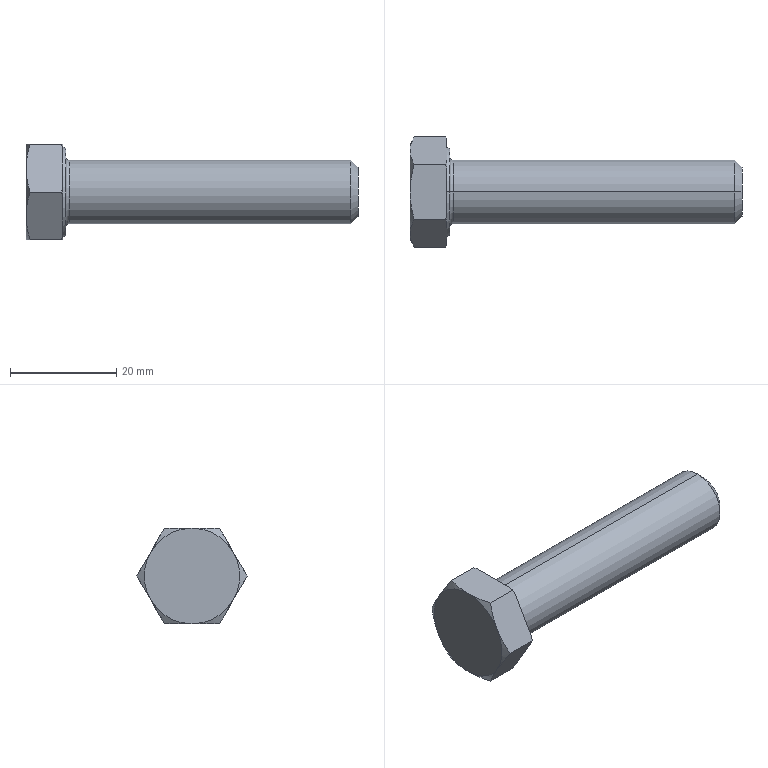Part | SolidWorks | features RevCut 4, Revolution 2, Chamfer 1, Extrusion 1, LPattern 1 | 1 solid | 30 faces | box 62.5 x 20.785 x 18 mm | volume 8250 mm3 | cone 16 | plane 10 | cylinder 2 | torus 2 | commonest cylinder face diameters 12 x2
STEP:
#1=CARTESIAN_POINT('',(8.1,0.,6.));
#2=VERTEX_POINT('',#1);
#3=CARTESIAN_POINT('',(8.1,0.,-6.));
#4=VERTEX_POINT('',#3);
#5=CARTESIAN_POINT('',(8.1,0.,0.));
#6=DIRECTION('',(-1.,0.,0.));
#7=DIRECTION('',(0.,0.,1.));
#8=AXIS2_PLACEMENT_3D('',#5,#6,#7);
#9=CIRCLE('',#8,6.);
#10=EDGE_CURVE('',#2,#4,#9,.T.);
#11=ORIENTED_EDGE('',*,*,#10,.F.);
#12=CARTESIAN_POINT('',(61.1,0.,6.));
#13=VERTEX_POINT('',#12);
#14=CARTESIAN_POINT('',(0.,0.,6.));
#15=DIRECTION('',(1.,0.,0.));
#16=VECTOR('',#15,1000.);
#17=LINE('',#14,#16);
#18=EDGE_CURVE('',#2,#13,#17,.T.);
#19=ORIENTED_EDGE('',*,*,#18,.T.);
#20=CARTESIAN_POINT('',(61.1,0.,-6.));
#21=VERTEX_POINT('',#20);
#22=CARTESIAN_POINT('',(61.1,0.,0.));
#23=DIRECTION('',(-1.,0.,0.));
#24=DIRECTION('',(0.,0.,-1.));
#25=AXIS2_PLACEMENT_3D('',#22,#23,#24);
#26=CIRCLE('',#25,6.);
#27=EDGE_CURVE('',#13,#21,#26,.T.);
#28=ORIENTED_EDGE('',*,*,#27,.T.);
#29=CARTESIAN_POINT('',(0.,0.,-6.));
#30=DIRECTION('',(1.,0.,0.));
#31=VECTOR('',#30,1000.);
#32=LINE('',#29,#31);
#33=EDGE_CURVE('',#4,#21,#32,.T.);
#34=ORIENTED_EDGE('',*,*,#33,.F.);
#35=EDGE_LOOP('',(#11,#19,#28,#34));
#36=FACE_OUTER_BOUND('',#35,.T.);
#37=CARTESIAN_POINT('',(0.,0.,0.));
#38=DIRECTION('',(1.,0.,0.));
#39=DIRECTION('',(0.,0.,-1.));
#40=AXIS2_PLACEMENT_3D('',#37,#38,#39);
#41=CYLINDRICAL_SURFACE('',#40,6.);
#42=ADVANCED_FACE('',(#36),#41,.T.);
#43=CARTESIAN_POINT('',(62.5,0.,-4.6));
#44=VERTEX_POINT('',#43);
#45=CARTESIAN_POINT('',(62.5,0.,4.6));
#46=VERTEX_POINT('',#45);
#47=CARTESIAN_POINT('',(62.5,0.,0.));
#48=DIRECTION('',(1.,0.,0.));
#49=DIRECTION('',(0.,0.,-1.));
#50=AXIS2_PLACEMENT_3D('',#47,#48,#49);
#51=CIRCLE('',#50,4.6);
#52=EDGE_CURVE('',#44,#46,#51,.T.);
#53=ORIENTED_EDGE('',*,*,#52,.F.);
#54=CARTESIAN_POINT('',(62.5,0.,-4.6));
#55=DIRECTION('',(-0.7071,0.,-0.7071));
#56=VECTOR('',#55,1000.);
#57=LINE('',#54,#56);
#58=EDGE_CURVE('',#44,#21,#57,.T.);
#59=ORIENTED_EDGE('',*,*,#58,.T.);
#60=ORIENTED_EDGE('',*,*,#27,.F.);
#61=CARTESIAN_POINT('',(62.5,0.,4.6));
#62=DIRECTION('',(-0.7071,0.,0.7071));
#63=VECTOR('',#62,1000.);
#64=LINE('',#61,#63);
#65=EDGE_CURVE('',#46,#13,#64,.T.);
#66=ORIENTED_EDGE('',*,*,#65,.F.);
#67=EDGE_LOOP('',(#53,#59,#60,#66));
#68=FACE_OUTER_BOUND('',#67,.T.);
#69=CARTESIAN_POINT('',(62.5,0.,0.));
#70=DIRECTION('',(-1.,0.,0.));
#71=DIRECTION('',(0.,0.,1.));
#72=AXIS2_PLACEMENT_3D('',#69,#70,#71);
#73=CONICAL_SURFACE('',#72,4.6,0.7854);
#74=ADVANCED_FACE('',(#68),#73,.T.);
#75=CARTESIAN_POINT('',(7.5,0.,-6.6));
#76=VERTEX_POINT('',#75);
#77=CARTESIAN_POINT('',(7.5,0.,6.6));
#78=VERTEX_POINT('',#77);
#79=CARTESIAN_POINT('',(7.5,0.,0.));
#80=DIRECTION('',(-1.,0.,0.));
#81=DIRECTION('',(0.,0.,1.));
#82=AXIS2_PLACEMENT_3D('',#79,#80,#81);
#83=CIRCLE('',#82,6.6);
#84=EDGE_CURVE('',#76,#78,#83,.T.);
#85=ORIENTED_EDGE('',*,*,#84,.F.);
#86=CARTESIAN_POINT('',(8.1,0.,-6.6));
#87=DIRECTION('',(0.,1.,0.));
#88=DIRECTION('',(-1.,0.,0.));
#89=AXIS2_PLACEMENT_3D('',#86,#87,#88);
#90=CIRCLE('',#89,0.6);
#91=EDGE_CURVE('',#76,#4,#90,.T.);
#92=ORIENTED_EDGE('',*,*,#91,.T.);
#93=CARTESIAN_POINT('',(8.1,0.,0.));
#94=DIRECTION('',(-1.,0.,0.));
#95=DIRECTION('',(0.,0.,1.));
#96=AXIS2_PLACEMENT_3D('',#93,#94,#95);
#97=CIRCLE('',#96,6.);
#98=EDGE_CURVE('',#4,#2,#97,.T.);
#99=ORIENTED_EDGE('',*,*,#98,.T.);
#100=CARTESIAN_POINT('',(8.1,0.,6.6));
#101=DIRECTION('',(0.,-1.,0.));
#102=DIRECTION('',(1.,0.,0.));
#103=AXIS2_PLACEMENT_3D('',#100,#101,#102);
#104=CIRCLE('',#103,0.6);
#105=EDGE_CURVE('',#78,#2,#104,.T.);
#106=ORIENTED_EDGE('',*,*,#105,.F.);
#107=EDGE_LOOP('',(#85,#92,#99,#106));
#108=FACE_OUTER_BOUND('',#107,.T.);
#109=CARTESIAN_POINT('',(8.1,0.,0.));
#110=DIRECTION('',(-1.,0.,0.));
#111=DIRECTION('',(0.,0.,1.));
#112=AXIS2_PLACEMENT_3D('',#109,#110,#111);
#113=TOROIDAL_SURFACE('',#112,6.6,0.6);
#114=ADVANCED_FACE('',(#108),#113,.F.);
#115=CARTESIAN_POINT('',(7.5,0.,8.177));
#116=VERTEX_POINT('',#115);
#117=CARTESIAN_POINT('',(7.5,0.,-8.177));
#118=VERTEX_POINT('',#117);
#119=CARTESIAN_POINT('',(7.5,0.,0.));
#120=DIRECTION('',(-1.,0.,0.));
#121=DIRECTION('',(0.,0.,1.));
#122=AXIS2_PLACEMENT_3D('',#119,#120,#121);
#123=CIRCLE('',#122,8.177);
#124=EDGE_CURVE('',#116,#118,#123,.T.);
#125=ORIENTED_EDGE('',*,*,#124,.T.);
#126=CARTESIAN_POINT('',(6.9,0.,-8.524));
#127=VERTEX_POINT('',#126);
#128=CARTESIAN_POINT('',(6.9,0.,-8.524));
#129=DIRECTION('',(-0.866,0.,-0.5));
#130=VECTOR('',#129,1000.);
#131=LINE('',#128,#130);
#132=EDGE_CURVE('',#118,#127,#131,.T.);
#133=ORIENTED_EDGE('',*,*,#132,.T.);
#134=CARTESIAN_POINT('',(6.9,0.,8.524));
#135=VERTEX_POINT('',#134);
#136=CARTESIAN_POINT('',(6.9,0.,0.));
#137=DIRECTION('',(-1.,0.,0.));
#138=DIRECTION('',(0.,0.,1.));
#139=AXIS2_PLACEMENT_3D('',#136,#137,#138);
#140=CIRCLE('',#139,8.524);
#141=EDGE_CURVE('',#135,#127,#140,.T.);
#142=ORIENTED_EDGE('',*,*,#141,.F.);
#143=CARTESIAN_POINT('',(6.9,0.,8.524));
#144=DIRECTION('',(-0.866,0.,0.5));
#145=VECTOR('',#144,1000.);
#146=LINE('',#143,#145);
#147=EDGE_CURVE('',#116,#135,#146,.T.);
#148=ORIENTED_EDGE('',*,*,#147,.F.);
#149=EDGE_LOOP('',(#125,#133,#142,#148));
#150=FACE_OUTER_BOUND('',#149,.T.);
#151=CARTESIAN_POINT('',(6.9,0.,0.));
#152=DIRECTION('',(-1.,0.,0.));
#153=DIRECTION('',(0.,0.,1.));
#154=AXIS2_PLACEMENT_3D('',#151,#152,#153);
#155=CONICAL_SURFACE('',#154,8.524,0.5236);
#156=ADVANCED_FACE('',(#150),#155,.T.);
#157=ORIENTED_EDGE('',*,*,#124,.F.);
#158=CARTESIAN_POINT('',(7.5,0.,0.));
#159=DIRECTION('',(-1.,0.,0.));
#160=DIRECTION('',(0.,0.,1.));
#161=AXIS2_PLACEMENT_3D('',#158,#159,#160);
#162=CIRCLE('',#161,8.177);
#163=EDGE_CURVE('',#118,#116,#162,.T.);
#164=ORIENTED_EDGE('',*,*,#163,.F.);
#165=EDGE_LOOP('',(#157,#164));
#166=FACE_OUTER_BOUND('',#165,.T.);
#167=CARTESIAN_POINT('',(7.5,0.,0.));
#168=DIRECTION('',(-1.,0.,0.));
#169=DIRECTION('',(0.,0.,1.));
#170=AXIS2_PLACEMENT_3D('',#167,#168,#169);
#171=CIRCLE('',#170,6.6);
#172=EDGE_CURVE('',#78,#76,#171,.T.);
#173=ORIENTED_EDGE('',*,*,#172,.T.);
#174=ORIENTED_EDGE('',*,*,#84,.T.);
#175=EDGE_LOOP('',(#173,#174));
#176=FACE_BOUND('',#175,.T.);
#177=CARTESIAN_POINT('',(7.5,0.,-18.));
#178=DIRECTION('',(1.,0.,0.));
#179=DIRECTION('',(0.,0.,-1.));
#180=AXIS2_PLACEMENT_3D('',#177,#178,#179);
#181=PLANE('',#180);
#182=ADVANCED_FACE('',(#166,#176),#181,.T.);
#183=CARTESIAN_POINT('',(6.9,5.57,-8.352));
#184=VERTEX_POINT('',#183);
#185=CARTESIAN_POINT('',(6.9,10.018,-0.6478));
#186=VERTEX_POINT('',#185);
#187=CARTESIAN_POINT('',(6.9,5.196,-9.));
#188=DIRECTION('',(0.,0.5,0.866));
#189=VECTOR('',#188,1000.);
#190=LINE('',#187,#189);
#191=EDGE_CURVE('',#184,#186,#190,.T.);
#192=ORIENTED_EDGE('',*,*,#191,.F.);
#193=CARTESIAN_POINT('',(6.696,5.196,-9.));
#194=VERTEX_POINT('',#193);
#195=CARTESIAN_POINT('',(6.696,5.196,-9.));
#196=CARTESIAN_POINT('',(6.768,5.321,-8.785));
#197=CARTESIAN_POINT('',(6.836,5.445,-8.569));
#198=CARTESIAN_POINT('',(6.9,5.57,-8.352));
#199=B_SPLINE_CURVE_WITH_KNOTS('',3,(#195,#196,#197,#198),.UNSPECIFIED.,.F.,.F.,(4,4),(0.000000238,0.0007696),.UNSPECIFIED.);
#200=EDGE_CURVE('',#194,#184,#199,.T.);
#201=ORIENTED_EDGE('',*,*,#200,.F.);
#202=CARTESIAN_POINT('',(0.8038,5.196,-9.));
#203=VERTEX_POINT('',#202);
#204=CARTESIAN_POINT('',(7.5,5.196,-9.));
#205=DIRECTION('',(-1.,0.,0.));
#206=VECTOR('',#205,1000.);
#207=LINE('',#204,#206);
#208=EDGE_CURVE('',#194,#203,#207,.T.);
#209=ORIENTED_EDGE('',*,*,#208,.T.);
#210=CARTESIAN_POINT('',(0.,7.794,-4.5));
#211=VERTEX_POINT('',#210);
#212=CARTESIAN_POINT('',(0.,7.794,-4.5));
#213=CARTESIAN_POINT('',(0.,7.574,-4.882));
#214=CARTESIAN_POINT('',(0.019,7.352,-5.266));
#215=CARTESIAN_POINT('',(0.09253,6.914,-6.024));
#216=CARTESIAN_POINT('',(0.147,6.697,-6.401));
#217=CARTESIAN_POINT('',(0.357,6.048,-7.525));
#218=CARTESIAN_POINT('',(0.5591,5.62,-8.266));
#219=CARTESIAN_POINT('',(0.8038,5.196,-9.));
#220=B_SPLINE_CURVE_WITH_KNOTS('',3,(#212,#213,#214,#215,#216,#217,#218,#219),.UNSPECIFIED.,.F.,.F.,(4,2,2,4),(0.005258,0.006567,0.007877,0.0105),.UNSPECIFIED.);
#221=EDGE_CURVE('',#211,#203,#220,.T.);
#222=ORIENTED_EDGE('',*,*,#221,.F.);
#223=CARTESIAN_POINT('',(0.8038,10.392,0.));
#224=VERTEX_POINT('',#223);
#225=CARTESIAN_POINT('',(0.8038,10.392,0.));
#226=CARTESIAN_POINT('',(0.5585,9.967,-0.7361));
#227=CARTESIAN_POINT('',(0.3563,9.539,-1.478));
#228=CARTESIAN_POINT('',(0.07661,8.674,-2.976));
#229=CARTESIAN_POINT('',(0.,8.237,-3.733));
#230=CARTESIAN_POINT('',(0.,7.794,-4.5));
#231=B_SPLINE_CURVE_WITH_KNOTS('',3,(#225,#226,#227,#228,#229,#230),.UNSPECIFIED.,.F.,.F.,(4,2,4),(0.000000238,0.002629,0.005258),.UNSPECIFIED.);
#232=EDGE_CURVE('',#224,#211,#231,.T.);
#233=ORIENTED_EDGE('',*,*,#232,.F.);
#234=CARTESIAN_POINT('',(6.696,10.392,0.));
#235=VERTEX_POINT('',#234);
#236=CARTESIAN_POINT('',(7.5,10.392,0.));
#237=DIRECTION('',(-1.,0.,0.));
#238=VECTOR('',#237,1000.);
#239=LINE('',#236,#238);
#240=EDGE_CURVE('',#235,#224,#239,.T.);
#241=ORIENTED_EDGE('',*,*,#240,.F.);
#242=CARTESIAN_POINT('',(6.9,10.018,-0.6478));
#243=CARTESIAN_POINT('',(6.836,10.143,-0.4313));
#244=CARTESIAN_POINT('',(6.768,10.268,-0.2154));
#245=CARTESIAN_POINT('',(6.696,10.392,0.));
#246=B_SPLINE_CURVE_WITH_KNOTS('',3,(#242,#243,#244,#245),.UNSPECIFIED.,.F.,.F.,(4,4),(0.009728,0.0105),.UNSPECIFIED.);
#247=EDGE_CURVE('',#186,#235,#246,.T.);
#248=ORIENTED_EDGE('',*,*,#247,.F.);
#249=EDGE_LOOP('',(#192,#201,#209,#222,#233,#241,#248));
#250=FACE_OUTER_BOUND('',#249,.T.);
#251=CARTESIAN_POINT('',(7.5,5.196,-9.));
#252=DIRECTION('',(0.,-0.866,0.5));
#253=DIRECTION('',(0.,-0.5,-0.866));
#254=AXIS2_PLACEMENT_3D('',#251,#252,#253);
#255=PLANE('',#254);
#256=ADVANCED_FACE('',(#250),#255,.F.);
#257=CARTESIAN_POINT('',(6.9,10.018,0.6478));
#258=VERTEX_POINT('',#257);
#259=CARTESIAN_POINT('',(6.9,5.57,8.352));
#260=VERTEX_POINT('',#259);
#261=CARTESIAN_POINT('',(6.9,10.392,0.));
#262=DIRECTION('',(0.,-0.5,0.866));
#263=VECTOR('',#262,1000.);
#264=LINE('',#261,#263);
#265=EDGE_CURVE('',#258,#260,#264,.T.);
#266=ORIENTED_EDGE('',*,*,#265,.F.);
#267=CARTESIAN_POINT('',(6.696,10.392,0.));
#268=CARTESIAN_POINT('',(6.768,10.268,0.2154));
#269=CARTESIAN_POINT('',(6.836,10.143,0.4314));
#270=CARTESIAN_POINT('',(6.9,10.018,0.6478));
#271=B_SPLINE_CURVE_WITH_KNOTS('',3,(#267,#268,#269,#270),.UNSPECIFIED.,.F.,.F.,(4,4),(0.000000238,0.0007696),.UNSPECIFIED.);
#272=EDGE_CURVE('',#235,#258,#271,.T.);
#273=ORIENTED_EDGE('',*,*,#272,.F.);
#274=ORIENTED_EDGE('',*,*,#240,.T.);
#275=CARTESIAN_POINT('',(0.,7.794,4.5));
#276=VERTEX_POINT('',#275);
#277=CARTESIAN_POINT('',(0.,7.794,4.5));
#278=CARTESIAN_POINT('',(0.,8.015,4.118));
#279=CARTESIAN_POINT('',(0.019,8.236,3.734));
#280=CARTESIAN_POINT('',(0.09253,8.674,2.976));
#281=CARTESIAN_POINT('',(0.147,8.892,2.599));
#282=CARTESIAN_POINT('',(0.357,9.541,1.475));
#283=CARTESIAN_POINT('',(0.5591,9.968,0.7343));
#284=CARTESIAN_POINT('',(0.8038,10.392,0.));
#285=B_SPLINE_CURVE_WITH_KNOTS('',3,(#277,#278,#279,#280,#281,#282,#283,#284),.UNSPECIFIED.,.F.,.F.,(4,2,2,4),(0.005258,0.006567,0.007877,0.0105),.UNSPECIFIED.);
#286=EDGE_CURVE('',#276,#224,#285,.T.);
#287=ORIENTED_EDGE('',*,*,#286,.F.);
#288=CARTESIAN_POINT('',(0.8038,5.196,9.));
#289=VERTEX_POINT('',#288);
#290=CARTESIAN_POINT('',(0.8038,5.196,9.));
#291=CARTESIAN_POINT('',(0.5585,5.621,8.264));
#292=CARTESIAN_POINT('',(0.3563,6.049,7.522));
#293=CARTESIAN_POINT('',(0.07661,6.914,6.024));
#294=CARTESIAN_POINT('',(0.,7.352,5.267));
#295=CARTESIAN_POINT('',(0.,7.794,4.5));
#296=B_SPLINE_CURVE_WITH_KNOTS('',3,(#290,#291,#292,#293,#294,#295),.UNSPECIFIED.,.F.,.F.,(4,2,4),(0.000000238,0.002629,0.005258),.UNSPECIFIED.);
#297=EDGE_CURVE('',#289,#276,#296,.T.);
#298=ORIENTED_EDGE('',*,*,#297,.F.);
#299=CARTESIAN_POINT('',(6.696,5.196,9.));
#300=VERTEX_POINT('',#299);
#301=CARTESIAN_POINT('',(7.5,5.196,9.));
#302=DIRECTION('',(-1.,0.,0.));
#303=VECTOR('',#302,1000.);
#304=LINE('',#301,#303);
#305=EDGE_CURVE('',#300,#289,#304,.T.);
#306=ORIENTED_EDGE('',*,*,#305,.F.);
#307=CARTESIAN_POINT('',(6.9,5.57,8.352));
#308=CARTESIAN_POINT('',(6.836,5.445,8.569));
#309=CARTESIAN_POINT('',(6.768,5.32,8.785));
#310=CARTESIAN_POINT('',(6.696,5.196,9.));
#311=B_SPLINE_CURVE_WITH_KNOTS('',3,(#307,#308,#309,#310),.UNSPECIFIED.,.F.,.F.,(4,4),(0.009728,0.0105),.UNSPECIFIED.);
#312=EDGE_CURVE('',#260,#300,#311,.T.);
#313=ORIENTED_EDGE('',*,*,#312,.F.);
#314=EDGE_LOOP('',(#266,#273,#274,#287,#298,#306,#313));
#315=FACE_OUTER_BOUND('',#314,.T.);
#316=CARTESIAN_POINT('',(7.5,10.392,0.));
#317=DIRECTION('',(0.,-0.866,-0.5));
#318=DIRECTION('',(0.,0.5,-0.866));
#319=AXIS2_PLACEMENT_3D('',#316,#317,#318);
#320=PLANE('',#319);
#321=ADVANCED_FACE('',(#315),#320,.F.);
#322=CARTESIAN_POINT('',(6.9,4.448,9.));
#323=VERTEX_POINT('',#322);
#324=CARTESIAN_POINT('',(6.9,-4.448,9.));
#325=VERTEX_POINT('',#324);
#326=CARTESIAN_POINT('',(6.9,5.196,9.));
#327=DIRECTION('',(0.,-1.,0.));
#328=VECTOR('',#327,1000.);
#329=LINE('',#326,#328);
#330=EDGE_CURVE('',#323,#325,#329,.T.);
#331=ORIENTED_EDGE('',*,*,#330,.F.);
#332=CARTESIAN_POINT('',(6.696,5.196,9.));
#333=CARTESIAN_POINT('',(6.768,4.948,9.));
#334=CARTESIAN_POINT('',(6.836,4.698,9.));
#335=CARTESIAN_POINT('',(6.9,4.448,9.));
#336=B_SPLINE_CURVE_WITH_KNOTS('',3,(#332,#333,#334,#335),.UNSPECIFIED.,.F.,.F.,(4,4),(0.02519,0.02597),.UNSPECIFIED.);
#337=EDGE_CURVE('',#300,#323,#336,.T.);
#338=ORIENTED_EDGE('',*,*,#337,.F.);
#339=ORIENTED_EDGE('',*,*,#305,.T.);
#340=CARTESIAN_POINT('',(0.,0.,9.));
#341=VERTEX_POINT('',#340);
#342=CARTESIAN_POINT('',(0.,0.,9.));
#343=CARTESIAN_POINT('',(0.,0.4401,9.));
#344=CARTESIAN_POINT('',(0.01885,0.8832,9.));
#345=CARTESIAN_POINT('',(0.09319,1.767,9.));
#346=CARTESIAN_POINT('',(0.1482,2.204,9.));
#347=CARTESIAN_POINT('',(0.3593,3.505,9.));
#348=CARTESIAN_POINT('',(0.5612,4.356,9.));
#349=CARTESIAN_POINT('',(0.8038,5.196,9.));
#350=B_SPLINE_CURVE_WITH_KNOTS('',3,(#342,#343,#344,#345,#346,#347,#348,#349),.UNSPECIFIED.,.F.,.F.,(4,2,2,4),(0.01498,0.0163,0.01761,0.02025),.UNSPECIFIED.);
#351=EDGE_CURVE('',#341,#289,#350,.T.);
#352=ORIENTED_EDGE('',*,*,#351,.F.);
#353=CARTESIAN_POINT('',(0.8038,-5.196,9.));
#354=VERTEX_POINT('',#353);
#355=CARTESIAN_POINT('',(0.8038,-5.196,9.));
#356=CARTESIAN_POINT('',(0.5595,-4.35,9.));
#357=CARTESIAN_POINT('',(0.3552,-3.485,9.));
#358=CARTESIAN_POINT('',(0.07569,-1.752,9.));
#359=CARTESIAN_POINT('',(0.,-0.8794,9.));
#360=CARTESIAN_POINT('',(0.,0.,9.));
#361=B_SPLINE_CURVE_WITH_KNOTS('',3,(#355,#356,#357,#358,#359,#360),.UNSPECIFIED.,.F.,.F.,(4,2,4),(0.00972,0.01235,0.01498),.UNSPECIFIED.);
#362=EDGE_CURVE('',#354,#341,#361,.T.);
#363=ORIENTED_EDGE('',*,*,#362,.F.);
#364=CARTESIAN_POINT('',(6.696,-5.196,9.));
#365=VERTEX_POINT('',#364);
#366=CARTESIAN_POINT('',(7.5,-5.196,9.));
#367=DIRECTION('',(-1.,0.,0.));
#368=VECTOR('',#367,1000.);
#369=LINE('',#366,#368);
#370=EDGE_CURVE('',#365,#354,#369,.T.);
#371=ORIENTED_EDGE('',*,*,#370,.F.);
#372=CARTESIAN_POINT('',(6.9,-4.448,9.));
#373=CARTESIAN_POINT('',(6.836,-4.699,9.));
#374=CARTESIAN_POINT('',(6.768,-4.948,9.));
#375=CARTESIAN_POINT('',(6.696,-5.196,9.));
#376=B_SPLINE_CURVE_WITH_KNOTS('',3,(#372,#373,#374,#375),.UNSPECIFIED.,.F.,.F.,(4,4),(0.03494,0.03571),.UNSPECIFIED.);
#377=EDGE_CURVE('',#325,#365,#376,.T.);
#378=ORIENTED_EDGE('',*,*,#377,.F.);
#379=EDGE_LOOP('',(#331,#338,#339,#352,#363,#371,#378));
#380=FACE_OUTER_BOUND('',#379,.T.);
#381=CARTESIAN_POINT('',(7.5,5.196,9.));
#382=DIRECTION('',(0.,0.,-1.));
#383=DIRECTION('',(0.,1.,0.));
#384=AXIS2_PLACEMENT_3D('',#381,#382,#383);
#385=PLANE('',#384);
#386=ADVANCED_FACE('',(#380),#385,.F.);
#387=CARTESIAN_POINT('',(6.9,-5.57,8.352));
#388=VERTEX_POINT('',#387);
#389=CARTESIAN_POINT('',(6.9,-10.018,0.6478));
#390=VERTEX_POINT('',#389);
#391=CARTESIAN_POINT('',(6.9,-10.392,0.));
#392=DIRECTION('',(0.,-0.5,-0.866));
#393=VECTOR('',#392,1000.);
#394=LINE('',#391,#393);
#395=EDGE_CURVE('',#388,#390,#394,.T.);
#396=ORIENTED_EDGE('',*,*,#395,.F.);
#397=CARTESIAN_POINT('',(6.696,-5.196,9.));
#398=CARTESIAN_POINT('',(6.768,-5.321,8.785));
#399=CARTESIAN_POINT('',(6.836,-5.445,8.569));
#400=CARTESIAN_POINT('',(6.9,-5.57,8.352));
#401=B_SPLINE_CURVE_WITH_KNOTS('',3,(#397,#398,#399,#400),.UNSPECIFIED.,.F.,.F.,(4,4),(0.000000238,0.0007696),.UNSPECIFIED.);
#402=EDGE_CURVE('',#365,#388,#401,.T.);
#403=ORIENTED_EDGE('',*,*,#402,.F.);
#404=ORIENTED_EDGE('',*,*,#370,.T.);
#405=CARTESIAN_POINT('',(0.,-7.794,4.5));
#406=VERTEX_POINT('',#405);
#407=CARTESIAN_POINT('',(0.,-7.794,4.5));
#408=CARTESIAN_POINT('',(0.,-7.574,4.882));
#409=CARTESIAN_POINT('',(0.019,-7.352,5.266));
#410=CARTESIAN_POINT('',(0.09253,-6.914,6.024));
#411=CARTESIAN_POINT('',(0.147,-6.697,6.401));
#412=CARTESIAN_POINT('',(0.357,-6.048,7.525));
#413=CARTESIAN_POINT('',(0.5591,-5.62,8.266));
#414=CARTESIAN_POINT('',(0.8038,-5.196,9.));
#415=B_SPLINE_CURVE_WITH_KNOTS('',3,(#407,#408,#409,#410,#411,#412,#413,#414),.UNSPECIFIED.,.F.,.F.,(4,2,2,4),(0.005258,0.006567,0.007877,0.0105),.UNSPECIFIED.);
#416=EDGE_CURVE('',#406,#354,#415,.T.);
#417=ORIENTED_EDGE('',*,*,#416,.F.);
#418=CARTESIAN_POINT('',(0.8038,-10.392,0.));
#419=VERTEX_POINT('',#418);
#420=CARTESIAN_POINT('',(0.8038,-10.392,0.));
#421=CARTESIAN_POINT('',(0.5585,-9.967,0.7361));
#422=CARTESIAN_POINT('',(0.3563,-9.539,1.478));
#423=CARTESIAN_POINT('',(0.07661,-8.674,2.976));
#424=CARTESIAN_POINT('',(0.,-8.237,3.733));
#425=CARTESIAN_POINT('',(0.,-7.794,4.5));
#426=B_SPLINE_CURVE_WITH_KNOTS('',3,(#420,#421,#422,#423,#424,#425),.UNSPECIFIED.,.F.,.F.,(4,2,4),(0.000000238,0.002629,0.005258),.UNSPECIFIED.);
#427=EDGE_CURVE('',#419,#406,#426,.T.);
#428=ORIENTED_EDGE('',*,*,#427,.F.);
#429=CARTESIAN_POINT('',(6.696,-10.392,0.));
#430=VERTEX_POINT('',#429);
#431=CARTESIAN_POINT('',(7.5,-10.392,0.));
#432=DIRECTION('',(-1.,0.,0.));
#433=VECTOR('',#432,1000.);
#434=LINE('',#431,#433);
#435=EDGE_CURVE('',#430,#419,#434,.T.);
#436=ORIENTED_EDGE('',*,*,#435,.F.);
#437=CARTESIAN_POINT('',(6.9,-10.018,0.6478));
#438=CARTESIAN_POINT('',(6.836,-10.143,0.4313));
#439=CARTESIAN_POINT('',(6.768,-10.268,0.2154));
#440=CARTESIAN_POINT('',(6.696,-10.392,0.));
#441=B_SPLINE_CURVE_WITH_KNOTS('',3,(#437,#438,#439,#440),.UNSPECIFIED.,.F.,.F.,(4,4),(0.009728,0.0105),.UNSPECIFIED.);
#442=EDGE_CURVE('',#390,#430,#441,.T.);
#443=ORIENTED_EDGE('',*,*,#442,.F.);
#444=EDGE_LOOP('',(#396,#403,#404,#417,#428,#436,#443));
#445=FACE_OUTER_BOUND('',#444,.T.);
#446=CARTESIAN_POINT('',(7.5,-10.392,0.));
#447=DIRECTION('',(0.,0.866,-0.5));
#448=DIRECTION('',(0.,0.5,0.866));
#449=AXIS2_PLACEMENT_3D('',#446,#447,#448);
#450=PLANE('',#449);
#451=ADVANCED_FACE('',(#445),#450,.F.);
#452=CARTESIAN_POINT('',(6.9,-10.018,-0.6478));
#453=VERTEX_POINT('',#452);
#454=CARTESIAN_POINT('',(6.9,-5.57,-8.352));
#455=VERTEX_POINT('',#454);
#456=CARTESIAN_POINT('',(6.9,-5.196,-9.));
#457=DIRECTION('',(0.,0.5,-0.866));
#458=VECTOR('',#457,1000.);
#459=LINE('',#456,#458);
#460=EDGE_CURVE('',#453,#455,#459,.T.);
#461=ORIENTED_EDGE('',*,*,#460,.F.);
#462=CARTESIAN_POINT('',(6.696,-10.392,0.));
#463=CARTESIAN_POINT('',(6.768,-10.268,-0.2154));
#464=CARTESIAN_POINT('',(6.836,-10.143,-0.4314));
#465=CARTESIAN_POINT('',(6.9,-10.018,-0.6478));
#466=B_SPLINE_CURVE_WITH_KNOTS('',3,(#462,#463,#464,#465),.UNSPECIFIED.,.F.,.F.,(4,4),(0.000000238,0.0007696),.UNSPECIFIED.);
#467=EDGE_CURVE('',#430,#453,#466,.T.);
#468=ORIENTED_EDGE('',*,*,#467,.F.);
#469=ORIENTED_EDGE('',*,*,#435,.T.);
#470=CARTESIAN_POINT('',(0.,-7.794,-4.5));
#471=VERTEX_POINT('',#470);
#472=CARTESIAN_POINT('',(0.,-7.794,-4.5));
#473=CARTESIAN_POINT('',(0.,-8.015,-4.118));
#474=CARTESIAN_POINT('',(0.019,-8.236,-3.734));
#475=CARTESIAN_POINT('',(0.09253,-8.674,-2.976));
#476=CARTESIAN_POINT('',(0.147,-8.892,-2.599));
#477=CARTESIAN_POINT('',(0.357,-9.541,-1.475));
#478=CARTESIAN_POINT('',(0.5591,-9.968,-0.7343));
#479=CARTESIAN_POINT('',(0.8038,-10.392,0.));
#480=B_SPLINE_CURVE_WITH_KNOTS('',3,(#472,#473,#474,#475,#476,#477,#478,#479),.UNSPECIFIED.,.F.,.F.,(4,2,2,4),(0.005258,0.006567,0.007877,0.0105),.UNSPECIFIED.);
#481=EDGE_CURVE('',#471,#419,#480,.T.);
#482=ORIENTED_EDGE('',*,*,#481,.F.);
#483=CARTESIAN_POINT('',(0.8038,-5.196,-9.));
#484=VERTEX_POINT('',#483);
#485=CARTESIAN_POINT('',(0.8038,-5.196,-9.));
#486=CARTESIAN_POINT('',(0.5585,-5.621,-8.264));
#487=CARTESIAN_POINT('',(0.3563,-6.049,-7.522));
#488=CARTESIAN_POINT('',(0.07661,-6.914,-6.024));
#489=CARTESIAN_POINT('',(0.,-7.352,-5.267));
#490=CARTESIAN_POINT('',(0.,-7.794,-4.5));
#491=B_SPLINE_CURVE_WITH_KNOTS('',3,(#485,#486,#487,#488,#489,#490),.UNSPECIFIED.,.F.,.F.,(4,2,4),(0.000000238,0.002629,0.005258),.UNSPECIFIED.);
#492=EDGE_CURVE('',#484,#471,#491,.T.);
#493=ORIENTED_EDGE('',*,*,#492,.F.);
#494=CARTESIAN_POINT('',(6.696,-5.196,-9.));
#495=VERTEX_POINT('',#494);
#496=CARTESIAN_POINT('',(7.5,-5.196,-9.));
#497=DIRECTION('',(-1.,0.,0.));
#498=VECTOR('',#497,1000.);
#499=LINE('',#496,#498);
#500=EDGE_CURVE('',#495,#484,#499,.T.);
#501=ORIENTED_EDGE('',*,*,#500,.F.);
#502=CARTESIAN_POINT('',(6.9,-5.57,-8.352));
#503=CARTESIAN_POINT('',(6.836,-5.445,-8.569));
#504=CARTESIAN_POINT('',(6.768,-5.32,-8.785));
#505=CARTESIAN_POINT('',(6.696,-5.196,-9.));
#506=B_SPLINE_CURVE_WITH_KNOTS('',3,(#502,#503,#504,#505),.UNSPECIFIED.,.F.,.F.,(4,4),(0.009728,0.0105),.UNSPECIFIED.);
#507=EDGE_CURVE('',#455,#495,#506,.T.);
#508=ORIENTED_EDGE('',*,*,#507,.F.);
#509=EDGE_LOOP('',(#461,#468,#469,#482,#493,#501,#508));
#510=FACE_OUTER_BOUND('',#509,.T.);
#511=CARTESIAN_POINT('',(7.5,-5.196,-9.));
#512=DIRECTION('',(0.,0.866,0.5));
#513=DIRECTION('',(0.,-0.5,0.866));
#514=AXIS2_PLACEMENT_3D('',#511,#512,#513);
#515=PLANE('',#514);
#516=ADVANCED_FACE('',(#510),#515,.F.);
#517=CARTESIAN_POINT('',(6.9,-4.448,-9.));
#518=VERTEX_POINT('',#517);
#519=CARTESIAN_POINT('',(6.9,4.448,-9.));
#520=VERTEX_POINT('',#519);
#521=CARTESIAN_POINT('',(6.9,5.196,-9.));
#522=DIRECTION('',(0.,1.,0.));
#523=VECTOR('',#522,1000.);
#524=LINE('',#521,#523);
#525=EDGE_CURVE('',#518,#520,#524,.T.);
#526=ORIENTED_EDGE('',*,*,#525,.F.);
#527=CARTESIAN_POINT('',(6.696,-5.196,-9.));
#528=CARTESIAN_POINT('',(6.768,-4.948,-9.));
#529=CARTESIAN_POINT('',(6.836,-4.699,-9.));
#530=CARTESIAN_POINT('',(6.9,-4.448,-9.));
#531=B_SPLINE_CURVE_WITH_KNOTS('',3,(#527,#528,#529,#530),.UNSPECIFIED.,.F.,.F.,(4,4),(0.00972,0.01049),.UNSPECIFIED.);
#532=EDGE_CURVE('',#495,#518,#531,.T.);
#533=ORIENTED_EDGE('',*,*,#532,.F.);
#534=ORIENTED_EDGE('',*,*,#500,.T.);
#535=CARTESIAN_POINT('',(0.,0.,-9.));
#536=VERTEX_POINT('',#535);
#537=CARTESIAN_POINT('',(0.,0.,-9.));
#538=CARTESIAN_POINT('',(0.,-0.8794,-9.));
#539=CARTESIAN_POINT('',(0.07569,-1.752,-9.));
#540=CARTESIAN_POINT('',(0.3552,-3.485,-9.));
#541=CARTESIAN_POINT('',(0.5595,-4.35,-9.));
#542=CARTESIAN_POINT('',(0.8038,-5.196,-9.));
#543=B_SPLINE_CURVE_WITH_KNOTS('',3,(#537,#538,#539,#540,#541,#542),.UNSPECIFIED.,.F.,.F.,(4,2,4),(0.03045,0.03308,0.03571),.UNSPECIFIED.);
#544=EDGE_CURVE('',#536,#484,#543,.T.);
#545=ORIENTED_EDGE('',*,*,#544,.F.);
#546=CARTESIAN_POINT('',(0.8038,5.196,-9.));
#547=CARTESIAN_POINT('',(0.5612,4.356,-9.));
#548=CARTESIAN_POINT('',(0.3593,3.505,-9.));
#549=CARTESIAN_POINT('',(0.1482,2.204,-9.));
#550=CARTESIAN_POINT('',(0.09319,1.767,-9.));
#551=CARTESIAN_POINT('',(0.01885,0.8832,-9.));
#552=CARTESIAN_POINT('',(0.,0.4401,-9.));
#553=CARTESIAN_POINT('',(0.,0.,-9.));
#554=B_SPLINE_CURVE_WITH_KNOTS('',3,(#546,#547,#548,#549,#550,#551,#552,#553),.UNSPECIFIED.,.F.,.F.,(4,2,2,4),(0.02519,0.02782,0.02914,0.03045),.UNSPECIFIED.);
#555=EDGE_CURVE('',#203,#536,#554,.T.);
#556=ORIENTED_EDGE('',*,*,#555,.F.);
#557=ORIENTED_EDGE('',*,*,#208,.F.);
#558=CARTESIAN_POINT('',(6.9,4.448,-9.));
#559=CARTESIAN_POINT('',(6.836,4.698,-9.));
#560=CARTESIAN_POINT('',(6.768,4.948,-9.));
#561=CARTESIAN_POINT('',(6.696,5.196,-9.));
#562=B_SPLINE_CURVE_WITH_KNOTS('',3,(#558,#559,#560,#561),.UNSPECIFIED.,.F.,.F.,(4,4),(0.01947,0.02025),.UNSPECIFIED.);
#563=EDGE_CURVE('',#520,#194,#562,.T.);
#564=ORIENTED_EDGE('',*,*,#563,.F.);
#565=EDGE_LOOP('',(#526,#533,#534,#545,#556,#557,#564));
#566=FACE_OUTER_BOUND('',#565,.T.);
#567=CARTESIAN_POINT('',(7.5,5.196,-9.));
#568=DIRECTION('',(0.,0.,1.));
#569=DIRECTION('',(0.,-1.,0.));
#570=AXIS2_PLACEMENT_3D('',#567,#568,#569);
#571=PLANE('',#570);
#572=ADVANCED_FACE('',(#566),#571,.F.);
#573=ORIENTED_EDGE('',*,*,#532,.T.);
#574=CARTESIAN_POINT('',(6.9,0.,0.));
#575=DIRECTION('',(-1.,0.,0.));
#576=DIRECTION('',(0.,0.,-1.));
#577=AXIS2_PLACEMENT_3D('',#574,#575,#576);
#578=CIRCLE('',#577,10.039);
#579=EDGE_CURVE('',#518,#455,#578,.T.);
#580=ORIENTED_EDGE('',*,*,#579,.T.);
#581=ORIENTED_EDGE('',*,*,#507,.T.);
#582=EDGE_LOOP('',(#573,#580,#581));
#583=FACE_OUTER_BOUND('',#582,.T.);
#584=CARTESIAN_POINT('',(3.809,0.,0.));
#585=DIRECTION('',(-1.,0.,0.));
#586=DIRECTION('',(0.,0.,1.));
#587=AXIS2_PLACEMENT_3D('',#584,#585,#586);
#588=CONICAL_SURFACE('',#587,15.392,1.047);
#589=ADVANCED_FACE('',(#583),#588,.T.);
#590=ORIENTED_EDGE('',*,*,#467,.T.);
#591=CARTESIAN_POINT('',(6.9,0.,0.));
#592=DIRECTION('',(-1.,0.,0.));
#593=DIRECTION('',(0.,0.,-1.));
#594=AXIS2_PLACEMENT_3D('',#591,#592,#593);
#595=CIRCLE('',#594,10.039);
#596=EDGE_CURVE('',#453,#390,#595,.T.);
#597=ORIENTED_EDGE('',*,*,#596,.T.);
#598=ORIENTED_EDGE('',*,*,#442,.T.);
#599=EDGE_LOOP('',(#590,#597,#598));
#600=FACE_OUTER_BOUND('',#599,.T.);
#601=CARTESIAN_POINT('',(3.809,0.,0.));
#602=DIRECTION('',(-1.,0.,0.));
#603=DIRECTION('',(0.,0.,1.));
#604=AXIS2_PLACEMENT_3D('',#601,#602,#603);
#605=CONICAL_SURFACE('',#604,15.392,1.047);
#606=ADVANCED_FACE('',(#600),#605,.T.);
#607=ORIENTED_EDGE('',*,*,#402,.T.);
#608=CARTESIAN_POINT('',(6.9,0.,0.));
#609=DIRECTION('',(-1.,0.,0.));
#610=DIRECTION('',(0.,0.,-1.));
#611=AXIS2_PLACEMENT_3D('',#608,#609,#610);
#612=CIRCLE('',#611,10.039);
#613=EDGE_CURVE('',#388,#325,#612,.T.);
#614=ORIENTED_EDGE('',*,*,#613,.T.);
#615=ORIENTED_EDGE('',*,*,#377,.T.);
#616=EDGE_LOOP('',(#607,#614,#615));
#617=FACE_OUTER_BOUND('',#616,.T.);
#618=CARTESIAN_POINT('',(3.809,0.,0.));
#619=DIRECTION('',(-1.,0.,0.));
#620=DIRECTION('',(0.,0.,1.));
#621=AXIS2_PLACEMENT_3D('',#618,#619,#620);
#622=CONICAL_SURFACE('',#621,15.392,1.047);
#623=ADVANCED_FACE('',(#617),#622,.T.);
#624=ORIENTED_EDGE('',*,*,#337,.T.);
#625=CARTESIAN_POINT('',(6.9,0.,0.));
#626=DIRECTION('',(-1.,0.,0.));
#627=DIRECTION('',(0.,0.,-1.));
#628=AXIS2_PLACEMENT_3D('',#625,#626,#627);
#629=CIRCLE('',#628,10.039);
#630=EDGE_CURVE('',#323,#260,#629,.T.);
#631=ORIENTED_EDGE('',*,*,#630,.T.);
#632=ORIENTED_EDGE('',*,*,#312,.T.);
#633=EDGE_LOOP('',(#624,#631,#632));
#634=FACE_OUTER_BOUND('',#633,.T.);
#635=CARTESIAN_POINT('',(3.809,0.,0.));
#636=DIRECTION('',(-1.,0.,0.));
#637=DIRECTION('',(0.,0.,1.));
#638=AXIS2_PLACEMENT_3D('',#635,#636,#637);
#639=CONICAL_SURFACE('',#638,15.392,1.047);
#640=ADVANCED_FACE('',(#634),#639,.T.);
#641=ORIENTED_EDGE('',*,*,#272,.T.);
#642=CARTESIAN_POINT('',(6.9,0.,0.));
#643=DIRECTION('',(-1.,0.,0.));
#644=DIRECTION('',(0.,0.,-1.));
#645=AXIS2_PLACEMENT_3D('',#642,#643,#644);
#646=CIRCLE('',#645,10.039);
#647=EDGE_CURVE('',#258,#186,#646,.T.);
#648=ORIENTED_EDGE('',*,*,#647,.T.);
#649=ORIENTED_EDGE('',*,*,#247,.T.);
#650=EDGE_LOOP('',(#641,#648,#649));
#651=FACE_OUTER_BOUND('',#650,.T.);
#652=CARTESIAN_POINT('',(3.809,0.,0.));
#653=DIRECTION('',(-1.,0.,0.));
#654=DIRECTION('',(0.,0.,1.));
#655=AXIS2_PLACEMENT_3D('',#652,#653,#654);
#656=CONICAL_SURFACE('',#655,15.392,1.047);
#657=ADVANCED_FACE('',(#651),#656,.T.);
#658=ORIENTED_EDGE('',*,*,#200,.T.);
#659=CARTESIAN_POINT('',(6.9,0.,0.));
#660=DIRECTION('',(-1.,0.,0.));
#661=DIRECTION('',(0.,0.,-1.));
#662=AXIS2_PLACEMENT_3D('',#659,#660,#661);
#663=CIRCLE('',#662,10.039);
#664=EDGE_CURVE('',#184,#520,#663,.T.);
#665=ORIENTED_EDGE('',*,*,#664,.T.);
#666=ORIENTED_EDGE('',*,*,#563,.T.);
#667=EDGE_LOOP('',(#658,#665,#666));
#668=FACE_OUTER_BOUND('',#667,.T.);
#669=CARTESIAN_POINT('',(3.809,0.,0.));
#670=DIRECTION('',(-1.,0.,0.));
#671=DIRECTION('',(0.,0.,1.));
#672=AXIS2_PLACEMENT_3D('',#669,#670,#671);
#673=CONICAL_SURFACE('',#672,15.392,1.047);
#674=ADVANCED_FACE('',(#668),#673,.T.);
#675=ORIENTED_EDGE('',*,*,#492,.T.);
#676=CARTESIAN_POINT('',(0.,0.,0.));
#677=DIRECTION('',(1.,0.,0.));
#678=DIRECTION('',(0.,0.,-1.));
#679=AXIS2_PLACEMENT_3D('',#676,#677,#678);
#680=CIRCLE('',#679,9.);
#681=EDGE_CURVE('',#471,#536,#680,.T.);
#682=ORIENTED_EDGE('',*,*,#681,.T.);
#683=ORIENTED_EDGE('',*,*,#544,.T.);
#684=EDGE_LOOP('',(#675,#682,#683));
#685=FACE_OUTER_BOUND('',#684,.T.);
#686=CARTESIAN_POINT('',(0.,0.,0.));
#687=DIRECTION('',(1.,0.,0.));
#688=DIRECTION('',(0.,0.,-1.));
#689=AXIS2_PLACEMENT_3D('',#686,#687,#688);
#690=CONICAL_SURFACE('',#689,9.,1.047);
#691=ADVANCED_FACE('',(#685),#690,.T.);
#692=ORIENTED_EDGE('',*,*,#427,.T.);
#693=CARTESIAN_POINT('',(0.,0.,0.));
#694=DIRECTION('',(1.,0.,0.));
#695=DIRECTION('',(0.,0.,-1.));
#696=AXIS2_PLACEMENT_3D('',#693,#694,#695);
#697=CIRCLE('',#696,9.);
#698=EDGE_CURVE('',#406,#471,#697,.T.);
#699=ORIENTED_EDGE('',*,*,#698,.T.);
#700=ORIENTED_EDGE('',*,*,#481,.T.);
#701=EDGE_LOOP('',(#692,#699,#700));
#702=FACE_OUTER_BOUND('',#701,.T.);
#703=CARTESIAN_POINT('',(0.,0.,0.));
#704=DIRECTION('',(1.,0.,0.));
#705=DIRECTION('',(0.,0.,-1.));
#706=AXIS2_PLACEMENT_3D('',#703,#704,#705);
#707=CONICAL_SURFACE('',#706,9.,1.047);
#708=ADVANCED_FACE('',(#702),#707,.T.);
#709=ORIENTED_EDGE('',*,*,#362,.T.);
#710=CARTESIAN_POINT('',(0.,0.,0.));
#711=DIRECTION('',(1.,0.,0.));
#712=DIRECTION('',(0.,0.,-1.));
#713=AXIS2_PLACEMENT_3D('',#710,#711,#712);
#714=CIRCLE('',#713,9.);
#715=EDGE_CURVE('',#341,#406,#714,.T.);
#716=ORIENTED_EDGE('',*,*,#715,.T.);
#717=ORIENTED_EDGE('',*,*,#416,.T.);
#718=EDGE_LOOP('',(#709,#716,#717));
#719=FACE_OUTER_BOUND('',#718,.T.);
#720=CARTESIAN_POINT('',(0.,0.,0.));
#721=DIRECTION('',(1.,0.,0.));
#722=DIRECTION('',(0.,0.,-1.));
#723=AXIS2_PLACEMENT_3D('',#720,#721,#722);
#724=CONICAL_SURFACE('',#723,9.,1.047);
#725=ADVANCED_FACE('',(#719),#724,.T.);
#726=ORIENTED_EDGE('',*,*,#351,.T.);
#727=ORIENTED_EDGE('',*,*,#297,.T.);
#728=CARTESIAN_POINT('',(0.,0.,0.));
#729=DIRECTION('',(-1.,0.,0.));
#730=DIRECTION('',(0.,0.,1.));
#731=AXIS2_PLACEMENT_3D('',#728,#729,#730);
#732=CIRCLE('',#731,9.);
#733=EDGE_CURVE('',#341,#276,#732,.T.);
#734=ORIENTED_EDGE('',*,*,#733,.F.);
#735=EDGE_LOOP('',(#726,#727,#734));
#736=FACE_OUTER_BOUND('',#735,.T.);
#737=CARTESIAN_POINT('',(0.,0.,0.));
#738=DIRECTION('',(1.,0.,0.));
#739=DIRECTION('',(0.,0.,-1.));
#740=AXIS2_PLACEMENT_3D('',#737,#738,#739);
#741=CONICAL_SURFACE('',#740,9.,1.047);
#742=ADVANCED_FACE('',(#736),#741,.T.);
#743=ORIENTED_EDGE('',*,*,#286,.T.);
#744=ORIENTED_EDGE('',*,*,#232,.T.);
#745=CARTESIAN_POINT('',(0.,0.,0.));
#746=DIRECTION('',(1.,0.,0.));
#747=DIRECTION('',(0.,0.,-1.));
#748=AXIS2_PLACEMENT_3D('',#745,#746,#747);
#749=CIRCLE('',#748,9.);
#750=EDGE_CURVE('',#211,#276,#749,.T.);
#751=ORIENTED_EDGE('',*,*,#750,.T.);
#752=EDGE_LOOP('',(#743,#744,#751));
#753=FACE_OUTER_BOUND('',#752,.T.);
#754=CARTESIAN_POINT('',(0.,0.,0.));
#755=DIRECTION('',(1.,0.,0.));
#756=DIRECTION('',(0.,0.,-1.));
#757=AXIS2_PLACEMENT_3D('',#754,#755,#756);
#758=CONICAL_SURFACE('',#757,9.,1.047);
#759=ADVANCED_FACE('',(#753),#758,.T.);
#760=ORIENTED_EDGE('',*,*,#221,.T.);
#761=ORIENTED_EDGE('',*,*,#555,.T.);
#762=CARTESIAN_POINT('',(0.,0.,0.));
#763=DIRECTION('',(1.,0.,0.));
#764=DIRECTION('',(0.,0.,-1.));
#765=AXIS2_PLACEMENT_3D('',#762,#763,#764);
#766=CIRCLE('',#765,9.);
#767=EDGE_CURVE('',#536,#211,#766,.T.);
#768=ORIENTED_EDGE('',*,*,#767,.T.);
#769=EDGE_LOOP('',(#760,#761,#768));
#770=FACE_OUTER_BOUND('',#769,.T.);
#771=CARTESIAN_POINT('',(0.,0.,0.));
#772=DIRECTION('',(1.,0.,0.));
#773=DIRECTION('',(0.,0.,-1.));
#774=AXIS2_PLACEMENT_3D('',#771,#772,#773);
#775=CONICAL_SURFACE('',#774,9.,1.047);
#776=ADVANCED_FACE('',(#770),#775,.T.);
#777=ORIENTED_EDGE('',*,*,#767,.F.);
#778=ORIENTED_EDGE('',*,*,#681,.F.);
#779=ORIENTED_EDGE('',*,*,#698,.F.);
#780=ORIENTED_EDGE('',*,*,#715,.F.);
#781=ORIENTED_EDGE('',*,*,#733,.T.);
#782=ORIENTED_EDGE('',*,*,#750,.F.);
#783=EDGE_LOOP('',(#777,#778,#779,#780,#781,#782));
#784=FACE_OUTER_BOUND('',#783,.T.);
#785=CARTESIAN_POINT('',(0.,0.,-18.));
#786=DIRECTION('',(1.,0.,0.));
#787=DIRECTION('',(0.,0.,-1.));
#788=AXIS2_PLACEMENT_3D('',#785,#786,#787);
#789=PLANE('',#788);
#790=ADVANCED_FACE('',(#784),#789,.F.);
#791=ORIENTED_EDGE('',*,*,#395,.T.);
#792=ORIENTED_EDGE('',*,*,#596,.F.);
#793=ORIENTED_EDGE('',*,*,#460,.T.);
#794=ORIENTED_EDGE('',*,*,#579,.F.);
#795=ORIENTED_EDGE('',*,*,#525,.T.);
#796=ORIENTED_EDGE('',*,*,#664,.F.);
#797=ORIENTED_EDGE('',*,*,#191,.T.);
#798=ORIENTED_EDGE('',*,*,#647,.F.);
#799=ORIENTED_EDGE('',*,*,#265,.T.);
#800=ORIENTED_EDGE('',*,*,#630,.F.);
#801=ORIENTED_EDGE('',*,*,#330,.T.);
#802=ORIENTED_EDGE('',*,*,#613,.F.);
#803=EDGE_LOOP('',(#791,#792,#793,#794,#795,#796,#797,#798,#799,#800,#801,#802));
#804=FACE_OUTER_BOUND('',#803,.T.);
#805=ORIENTED_EDGE('',*,*,#141,.T.);
#806=CARTESIAN_POINT('',(6.9,0.,0.));
#807=DIRECTION('',(-1.,0.,0.));
#808=DIRECTION('',(0.,0.,1.));
#809=AXIS2_PLACEMENT_3D('',#806,#807,#808);
#810=CIRCLE('',#809,8.524);
#811=EDGE_CURVE('',#127,#135,#810,.T.);
#812=ORIENTED_EDGE('',*,*,#811,.T.);
#813=EDGE_LOOP('',(#805,#812));
#814=FACE_BOUND('',#813,.T.);
#815=CARTESIAN_POINT('',(6.9,8.524,0.));
#816=DIRECTION('',(1.,0.,0.));
#817=DIRECTION('',(0.,0.,-1.));
#818=AXIS2_PLACEMENT_3D('',#815,#816,#817);
#819=PLANE('',#818);
#820=ADVANCED_FACE('',(#804,#814),#819,.T.);
#821=ORIENTED_EDGE('',*,*,#132,.F.);
#822=ORIENTED_EDGE('',*,*,#163,.T.);
#823=ORIENTED_EDGE('',*,*,#147,.T.);
#824=ORIENTED_EDGE('',*,*,#811,.F.);
#825=EDGE_LOOP('',(#821,#822,#823,#824));
#826=FACE_OUTER_BOUND('',#825,.T.);
#827=CARTESIAN_POINT('',(6.9,0.,0.));
#828=DIRECTION('',(-1.,0.,0.));
#829=DIRECTION('',(0.,0.,1.));
#830=AXIS2_PLACEMENT_3D('',#827,#828,#829);
#831=CONICAL_SURFACE('',#830,8.524,0.5236);
#832=ADVANCED_FACE('',(#826),#831,.T.);
#833=ORIENTED_EDGE('',*,*,#91,.F.);
#834=ORIENTED_EDGE('',*,*,#172,.F.);
#835=ORIENTED_EDGE('',*,*,#105,.T.);
#836=ORIENTED_EDGE('',*,*,#10,.T.);
#837=EDGE_LOOP('',(#833,#834,#835,#836));
#838=FACE_OUTER_BOUND('',#837,.T.);
#839=CARTESIAN_POINT('',(8.1,0.,0.));
#840=DIRECTION('',(-1.,0.,0.));
#841=DIRECTION('',(0.,0.,1.));
#842=AXIS2_PLACEMENT_3D('',#839,#840,#841);
#843=TOROIDAL_SURFACE('',#842,6.6,0.6);
#844=ADVANCED_FACE('',(#838),#843,.F.);
#845=CARTESIAN_POINT('',(62.5,0.,0.));
#846=DIRECTION('',(1.,0.,0.));
#847=DIRECTION('',(0.,0.,-1.));
#848=AXIS2_PLACEMENT_3D('',#845,#846,#847);
#849=CIRCLE('',#848,4.6);
#850=EDGE_CURVE('',#46,#44,#849,.T.);
#851=ORIENTED_EDGE('',*,*,#850,.T.);
#852=ORIENTED_EDGE('',*,*,#52,.T.);
#853=EDGE_LOOP('',(#851,#852));
#854=FACE_OUTER_BOUND('',#853,.T.);
#855=CARTESIAN_POINT('',(62.5,0.,0.));
#856=DIRECTION('',(1.,0.,0.));
#857=DIRECTION('',(0.,0.,-1.));
#858=AXIS2_PLACEMENT_3D('',#855,#856,#857);
#859=PLANE('',#858);
#860=ADVANCED_FACE('',(#854),#859,.T.);
#861=ORIENTED_EDGE('',*,*,#58,.F.);
#862=ORIENTED_EDGE('',*,*,#850,.F.);
#863=ORIENTED_EDGE('',*,*,#65,.T.);
#864=CARTESIAN_POINT('',(61.1,0.,0.));
#865=DIRECTION('',(-1.,0.,0.));
#866=DIRECTION('',(0.,0.,-1.));
#867=AXIS2_PLACEMENT_3D('',#864,#865,#866);
#868=CIRCLE('',#867,6.);
#869=EDGE_CURVE('',#21,#13,#868,.T.);
#870=ORIENTED_EDGE('',*,*,#869,.F.);
#871=EDGE_LOOP('',(#861,#862,#863,#870));
#872=FACE_OUTER_BOUND('',#871,.T.);
#873=CARTESIAN_POINT('',(62.5,0.,0.));
#874=DIRECTION('',(-1.,0.,0.));
#875=DIRECTION('',(0.,0.,1.));
#876=AXIS2_PLACEMENT_3D('',#873,#874,#875);
#877=CONICAL_SURFACE('',#876,4.6,0.7854);
#878=ADVANCED_FACE('',(#872),#877,.T.);
#879=ORIENTED_EDGE('',*,*,#18,.F.);
#880=ORIENTED_EDGE('',*,*,#98,.F.);
#881=ORIENTED_EDGE('',*,*,#33,.T.);
#882=ORIENTED_EDGE('',*,*,#869,.T.);
#883=EDGE_LOOP('',(#879,#880,#881,#882));
#884=FACE_OUTER_BOUND('',#883,.T.);
#885=CARTESIAN_POINT('',(0.,0.,0.));
#886=DIRECTION('',(1.,0.,0.));
#887=DIRECTION('',(0.,0.,-1.));
#888=AXIS2_PLACEMENT_3D('',#885,#886,#887);
#889=CYLINDRICAL_SURFACE('',#888,6.);
#890=ADVANCED_FACE('',(#884),#889,.T.);
#891=CLOSED_SHELL('',(#42,#74,#114,#156,#182,#256,#321,#386,#451,#516,#572,#589,#606,#623,#640,#657,#674,#691,#708,#725,#742,#759,#776,#790,#820,#832,#844,#860,#878,#890));
#892=MANIFOLD_SOLID_BREP('',#891);
#893=CARTESIAN_POINT('',(0.,0.,0.));
#894=DIRECTION('',(0.,0.,1.));
#895=DIRECTION('',(1.,0.,0.));
#896=AXIS2_PLACEMENT_3D('',#893,#894,#895);
#897=(LENGTH_UNIT()NAMED_UNIT(*)SI_UNIT(.MILLI.,.METRE.));
#898=UNCERTAINTY_MEASURE_WITH_UNIT(LENGTH_MEASURE(0.00001),#897,'','');
#899=(NAMED_UNIT(*)PLANE_ANGLE_UNIT()SI_UNIT($,.RADIAN.));
#900=(NAMED_UNIT(*)SI_UNIT($,.STERADIAN.)SOLID_ANGLE_UNIT());
#901=(GEOMETRIC_REPRESENTATION_CONTEXT(3)GLOBAL_UNCERTAINTY_ASSIGNED_CONTEXT((#898))GLOBAL_UNIT_ASSIGNED_CONTEXT((#897,#899,#900))REPRESENTATION_CONTEXT('',''));
#902=ADVANCED_BREP_SHAPE_REPRESENTATION('',(#892,#896),#901);